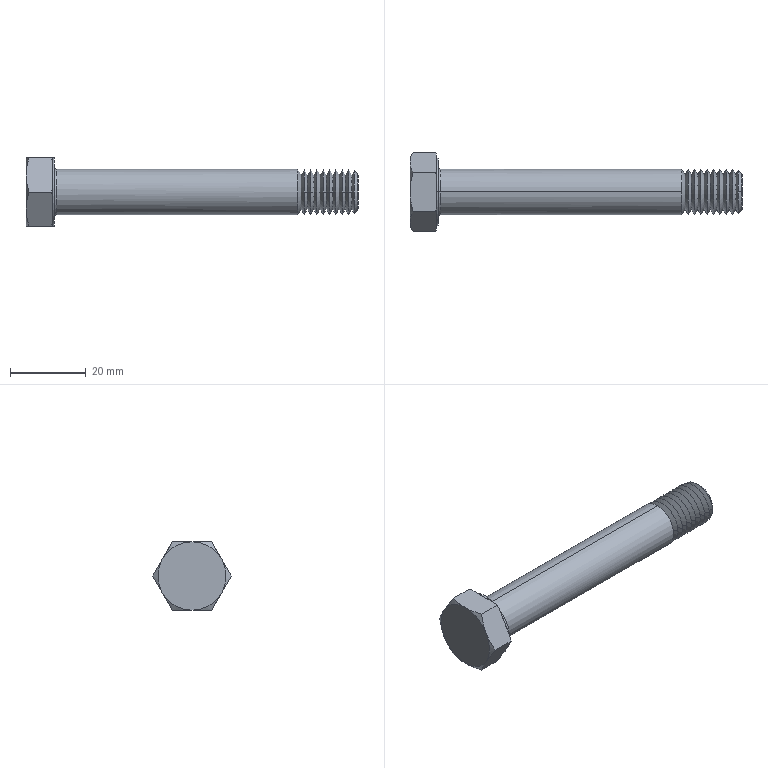Part | SolidWorks | features RevCut 4, Chamfer 1, Extrusion 1, Fillet 1, LPattern 1, Revolution 1 | 1 solid | 73 faces | box 87.5 x 20.785 x 18 mm | volume 10692 mm3 | cone 52 | plane 15 | cylinder 4 | torus 2 | commonest cylinder face diameters 12 x2 18 x2